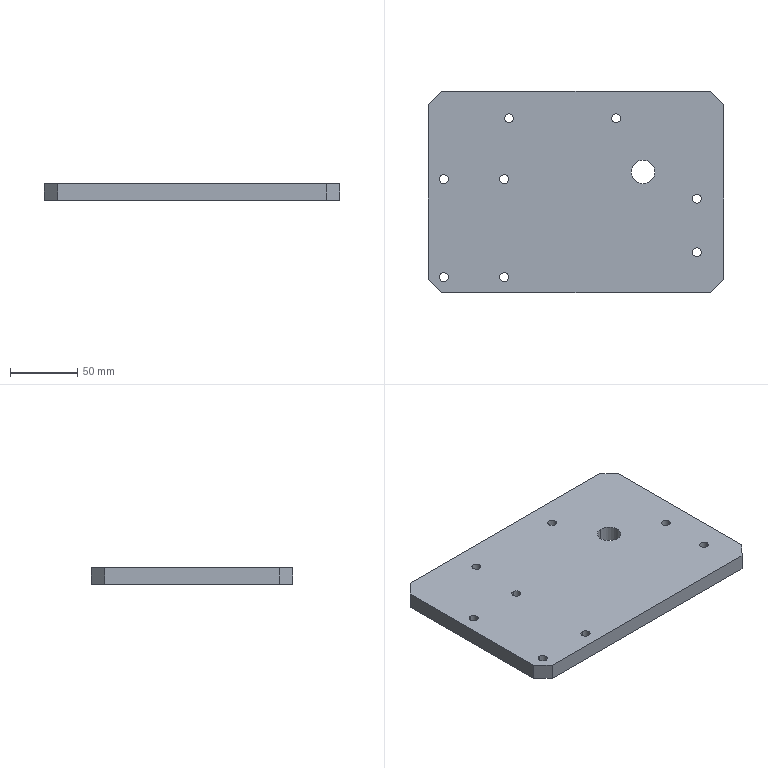Part | SolidWorks | features BaseBody 1 | 1 solid | 40 faces | box 220 x 150 x 12 mm | volume 385674 mm3 | cylinder 26 | plane 14 | commonest cylinder face diameters 6.6 x8 6.8 x8 11 x8 17.5 x2
STEP:
#1=CARTESIAN_POINT('',(349.217,495.647,-547.5));
#2=VERTEX_POINT('',#1);
#3=CARTESIAN_POINT('',(355.817,495.647,-547.5));
#4=VERTEX_POINT('',#3);
#5=CARTESIAN_POINT('',(352.517,495.647,-547.5));
#6=DIRECTION('',(0.,0.,1.));
#7=DIRECTION('',(-1.,0.,0.));
#8=AXIS2_PLACEMENT_3D('',#5,#6,#7);
#9=CIRCLE('',#8,3.3);
#10=EDGE_CURVE('',#2,#4,#9,.T.);
#11=ORIENTED_EDGE('',*,*,#10,.T.);
#12=CARTESIAN_POINT('',(355.817,495.647,-552.7));
#13=VERTEX_POINT('',#12);
#14=CARTESIAN_POINT('',(355.817,495.647,-559.5));
#15=DIRECTION('',(0.,0.,-1.));
#16=VECTOR('',#15,1000.);
#17=LINE('',#14,#16);
#18=EDGE_CURVE('',#4,#13,#17,.T.);
#19=ORIENTED_EDGE('',*,*,#18,.T.);
#20=CARTESIAN_POINT('',(349.217,495.647,-552.7));
#21=VERTEX_POINT('',#20);
#22=CARTESIAN_POINT('',(352.517,495.647,-552.7));
#23=DIRECTION('',(0.,0.,1.));
#24=DIRECTION('',(-1.,0.,0.));
#25=AXIS2_PLACEMENT_3D('',#22,#23,#24);
#26=CIRCLE('',#25,3.3);
#27=EDGE_CURVE('',#21,#13,#26,.T.);
#28=ORIENTED_EDGE('',*,*,#27,.F.);
#29=CARTESIAN_POINT('',(349.217,495.647,-559.5));
#30=DIRECTION('',(0.,0.,-1.));
#31=VECTOR('',#30,1000.);
#32=LINE('',#29,#31);
#33=EDGE_CURVE('',#2,#21,#32,.T.);
#34=ORIENTED_EDGE('',*,*,#33,.F.);
#35=EDGE_LOOP('',(#11,#19,#28,#34));
#36=FACE_OUTER_BOUND('',#35,.T.);
#37=CARTESIAN_POINT('',(352.517,495.647,-559.5));
#38=DIRECTION('',(0.,0.,-1.));
#39=DIRECTION('',(-1.,0.,0.));
#40=AXIS2_PLACEMENT_3D('',#37,#38,#39);
#41=CYLINDRICAL_SURFACE('',#40,3.3);
#42=ADVANCED_FACE('',(#36),#41,.F.);
#43=CARTESIAN_POINT('',(429.217,495.647,-547.5));
#44=VERTEX_POINT('',#43);
#45=CARTESIAN_POINT('',(435.817,495.647,-547.5));
#46=VERTEX_POINT('',#45);
#47=CARTESIAN_POINT('',(432.517,495.647,-547.5));
#48=DIRECTION('',(0.,0.,1.));
#49=DIRECTION('',(-1.,0.,0.));
#50=AXIS2_PLACEMENT_3D('',#47,#48,#49);
#51=CIRCLE('',#50,3.3);
#52=EDGE_CURVE('',#44,#46,#51,.T.);
#53=ORIENTED_EDGE('',*,*,#52,.T.);
#54=CARTESIAN_POINT('',(435.817,495.647,-552.7));
#55=VERTEX_POINT('',#54);
#56=CARTESIAN_POINT('',(435.817,495.647,-559.5));
#57=DIRECTION('',(0.,0.,-1.));
#58=VECTOR('',#57,1000.);
#59=LINE('',#56,#58);
#60=EDGE_CURVE('',#46,#55,#59,.T.);
#61=ORIENTED_EDGE('',*,*,#60,.T.);
#62=CARTESIAN_POINT('',(429.217,495.647,-552.7));
#63=VERTEX_POINT('',#62);
#64=CARTESIAN_POINT('',(432.517,495.647,-552.7));
#65=DIRECTION('',(0.,0.,1.));
#66=DIRECTION('',(-1.,0.,0.));
#67=AXIS2_PLACEMENT_3D('',#64,#65,#66);
#68=CIRCLE('',#67,3.3);
#69=EDGE_CURVE('',#63,#55,#68,.T.);
#70=ORIENTED_EDGE('',*,*,#69,.F.);
#71=CARTESIAN_POINT('',(429.217,495.647,-559.5));
#72=DIRECTION('',(0.,0.,-1.));
#73=VECTOR('',#72,1000.);
#74=LINE('',#71,#73);
#75=EDGE_CURVE('',#44,#63,#74,.T.);
#76=ORIENTED_EDGE('',*,*,#75,.F.);
#77=EDGE_LOOP('',(#53,#61,#70,#76));
#78=FACE_OUTER_BOUND('',#77,.T.);
#79=CARTESIAN_POINT('',(432.517,495.647,-559.5));
#80=DIRECTION('',(0.,0.,-1.));
#81=DIRECTION('',(-1.,0.,0.));
#82=AXIS2_PLACEMENT_3D('',#79,#80,#81);
#83=CYLINDRICAL_SURFACE('',#82,3.3);
#84=ADVANCED_FACE('',(#78),#83,.F.);
#85=CARTESIAN_POINT('',(489.217,395.647,-547.5));
#86=VERTEX_POINT('',#85);
#87=CARTESIAN_POINT('',(495.817,395.647,-547.5));
#88=VERTEX_POINT('',#87);
#89=CARTESIAN_POINT('',(492.517,395.647,-547.5));
#90=DIRECTION('',(0.,0.,1.));
#91=DIRECTION('',(-1.,0.,0.));
#92=AXIS2_PLACEMENT_3D('',#89,#90,#91);
#93=CIRCLE('',#92,3.3);
#94=EDGE_CURVE('',#86,#88,#93,.T.);
#95=ORIENTED_EDGE('',*,*,#94,.T.);
#96=CARTESIAN_POINT('',(495.817,395.647,-552.7));
#97=VERTEX_POINT('',#96);
#98=CARTESIAN_POINT('',(495.817,395.647,-559.5));
#99=DIRECTION('',(0.,0.,-1.));
#100=VECTOR('',#99,1000.);
#101=LINE('',#98,#100);
#102=EDGE_CURVE('',#88,#97,#101,.T.);
#103=ORIENTED_EDGE('',*,*,#102,.T.);
#104=CARTESIAN_POINT('',(489.217,395.647,-552.7));
#105=VERTEX_POINT('',#104);
#106=CARTESIAN_POINT('',(492.517,395.647,-552.7));
#107=DIRECTION('',(0.,0.,1.));
#108=DIRECTION('',(-1.,0.,0.));
#109=AXIS2_PLACEMENT_3D('',#106,#107,#108);
#110=CIRCLE('',#109,3.3);
#111=EDGE_CURVE('',#105,#97,#110,.T.);
#112=ORIENTED_EDGE('',*,*,#111,.F.);
#113=CARTESIAN_POINT('',(489.217,395.647,-559.5));
#114=DIRECTION('',(0.,0.,-1.));
#115=VECTOR('',#114,1000.);
#116=LINE('',#113,#115);
#117=EDGE_CURVE('',#86,#105,#116,.T.);
#118=ORIENTED_EDGE('',*,*,#117,.F.);
#119=EDGE_LOOP('',(#95,#103,#112,#118));
#120=FACE_OUTER_BOUND('',#119,.T.);
#121=CARTESIAN_POINT('',(492.517,395.647,-559.5));
#122=DIRECTION('',(0.,0.,-1.));
#123=DIRECTION('',(-1.,0.,0.));
#124=AXIS2_PLACEMENT_3D('',#121,#122,#123);
#125=CYLINDRICAL_SURFACE('',#124,3.3);
#126=ADVANCED_FACE('',(#120),#125,.F.);
#127=CARTESIAN_POINT('',(489.217,435.647,-547.5));
#128=VERTEX_POINT('',#127);
#129=CARTESIAN_POINT('',(495.817,435.647,-547.5));
#130=VERTEX_POINT('',#129);
#131=CARTESIAN_POINT('',(492.517,435.647,-547.5));
#132=DIRECTION('',(0.,0.,1.));
#133=DIRECTION('',(-1.,0.,0.));
#134=AXIS2_PLACEMENT_3D('',#131,#132,#133);
#135=CIRCLE('',#134,3.3);
#136=EDGE_CURVE('',#128,#130,#135,.T.);
#137=ORIENTED_EDGE('',*,*,#136,.T.);
#138=CARTESIAN_POINT('',(495.817,435.647,-552.7));
#139=VERTEX_POINT('',#138);
#140=CARTESIAN_POINT('',(495.817,435.647,-559.5));
#141=DIRECTION('',(0.,0.,-1.));
#142=VECTOR('',#141,1000.);
#143=LINE('',#140,#142);
#144=EDGE_CURVE('',#130,#139,#143,.T.);
#145=ORIENTED_EDGE('',*,*,#144,.T.);
#146=CARTESIAN_POINT('',(489.217,435.647,-552.7));
#147=VERTEX_POINT('',#146);
#148=CARTESIAN_POINT('',(492.517,435.647,-552.7));
#149=DIRECTION('',(0.,0.,1.));
#150=DIRECTION('',(-1.,0.,0.));
#151=AXIS2_PLACEMENT_3D('',#148,#149,#150);
#152=CIRCLE('',#151,3.3);
#153=EDGE_CURVE('',#147,#139,#152,.T.);
#154=ORIENTED_EDGE('',*,*,#153,.F.);
#155=CARTESIAN_POINT('',(489.217,435.647,-559.5));
#156=DIRECTION('',(0.,0.,-1.));
#157=VECTOR('',#156,1000.);
#158=LINE('',#155,#157);
#159=EDGE_CURVE('',#128,#147,#158,.T.);
#160=ORIENTED_EDGE('',*,*,#159,.F.);
#161=EDGE_LOOP('',(#137,#145,#154,#160));
#162=FACE_OUTER_BOUND('',#161,.T.);
#163=CARTESIAN_POINT('',(492.517,435.647,-559.5));
#164=DIRECTION('',(0.,0.,-1.));
#165=DIRECTION('',(-1.,0.,0.));
#166=AXIS2_PLACEMENT_3D('',#163,#164,#165);
#167=CYLINDRICAL_SURFACE('',#166,3.3);
#168=ADVANCED_FACE('',(#162),#167,.F.);
#169=CARTESIAN_POINT('',(452.517,464.397,-547.5));
#170=VERTEX_POINT('',#169);
#171=CARTESIAN_POINT('',(452.517,446.897,-547.5));
#172=VERTEX_POINT('',#171);
#173=CARTESIAN_POINT('',(452.517,455.647,-547.5));
#174=DIRECTION('',(0.,0.,1.));
#175=DIRECTION('',(0.,1.,0.));
#176=AXIS2_PLACEMENT_3D('',#173,#174,#175);
#177=CIRCLE('',#176,8.75);
#178=EDGE_CURVE('',#170,#172,#177,.T.);
#179=ORIENTED_EDGE('',*,*,#178,.T.);
#180=CARTESIAN_POINT('',(452.517,446.897,-559.5));
#181=VERTEX_POINT('',#180);
#182=CARTESIAN_POINT('',(452.517,446.897,-559.5));
#183=DIRECTION('',(0.,0.,-1.));
#184=VECTOR('',#183,1000.);
#185=LINE('',#182,#184);
#186=EDGE_CURVE('',#172,#181,#185,.T.);
#187=ORIENTED_EDGE('',*,*,#186,.T.);
#188=CARTESIAN_POINT('',(452.517,464.397,-559.5));
#189=VERTEX_POINT('',#188);
#190=CARTESIAN_POINT('',(452.517,455.647,-559.5));
#191=DIRECTION('',(0.,0.,1.));
#192=DIRECTION('',(0.,1.,0.));
#193=AXIS2_PLACEMENT_3D('',#190,#191,#192);
#194=CIRCLE('',#193,8.75);
#195=EDGE_CURVE('',#189,#181,#194,.T.);
#196=ORIENTED_EDGE('',*,*,#195,.F.);
#197=CARTESIAN_POINT('',(452.517,464.397,-559.5));
#198=DIRECTION('',(0.,0.,-1.));
#199=VECTOR('',#198,1000.);
#200=LINE('',#197,#199);
#201=EDGE_CURVE('',#170,#189,#200,.T.);
#202=ORIENTED_EDGE('',*,*,#201,.F.);
#203=EDGE_LOOP('',(#179,#187,#196,#202));
#204=FACE_OUTER_BOUND('',#203,.T.);
#205=CARTESIAN_POINT('',(452.517,455.647,-559.5));
#206=DIRECTION('',(0.,0.,-1.));
#207=DIRECTION('',(0.,1.,0.));
#208=AXIS2_PLACEMENT_3D('',#205,#206,#207);
#209=CYLINDRICAL_SURFACE('',#208,8.75);
#210=ADVANCED_FACE('',(#204),#209,.F.);
#211=CARTESIAN_POINT('',(304.017,380.547,-547.5));
#212=VERTEX_POINT('',#211);
#213=CARTESIAN_POINT('',(304.017,373.747,-547.5));
#214=VERTEX_POINT('',#213);
#215=CARTESIAN_POINT('',(304.017,377.147,-547.5));
#216=DIRECTION('',(0.,0.,1.));
#217=DIRECTION('',(0.,1.,0.));
#218=AXIS2_PLACEMENT_3D('',#215,#216,#217);
#219=CIRCLE('',#218,3.4);
#220=EDGE_CURVE('',#212,#214,#219,.T.);
#221=ORIENTED_EDGE('',*,*,#220,.T.);
#222=CARTESIAN_POINT('',(304.017,373.747,-559.5));
#223=VERTEX_POINT('',#222);
#224=CARTESIAN_POINT('',(304.017,373.747,-559.5));
#225=DIRECTION('',(0.,0.,-1.));
#226=VECTOR('',#225,1000.);
#227=LINE('',#224,#226);
#228=EDGE_CURVE('',#214,#223,#227,.T.);
#229=ORIENTED_EDGE('',*,*,#228,.T.);
#230=CARTESIAN_POINT('',(304.017,380.547,-559.5));
#231=VERTEX_POINT('',#230);
#232=CARTESIAN_POINT('',(304.017,377.147,-559.5));
#233=DIRECTION('',(0.,0.,1.));
#234=DIRECTION('',(0.,1.,0.));
#235=AXIS2_PLACEMENT_3D('',#232,#233,#234);
#236=CIRCLE('',#235,3.4);
#237=EDGE_CURVE('',#231,#223,#236,.T.);
#238=ORIENTED_EDGE('',*,*,#237,.F.);
#239=CARTESIAN_POINT('',(304.017,380.547,-559.5));
#240=DIRECTION('',(0.,0.,-1.));
#241=VECTOR('',#240,1000.);
#242=LINE('',#239,#241);
#243=EDGE_CURVE('',#212,#231,#242,.T.);
#244=ORIENTED_EDGE('',*,*,#243,.F.);
#245=EDGE_LOOP('',(#221,#229,#238,#244));
#246=FACE_OUTER_BOUND('',#245,.T.);
#247=CARTESIAN_POINT('',(304.017,377.147,-559.5));
#248=DIRECTION('',(0.,0.,-1.));
#249=DIRECTION('',(0.,1.,0.));
#250=AXIS2_PLACEMENT_3D('',#247,#248,#249);
#251=CYLINDRICAL_SURFACE('',#250,3.4);
#252=ADVANCED_FACE('',(#246),#251,.F.);
#253=CARTESIAN_POINT('',(349.017,380.547,-547.5));
#254=VERTEX_POINT('',#253);
#255=CARTESIAN_POINT('',(349.017,373.747,-547.5));
#256=VERTEX_POINT('',#255);
#257=CARTESIAN_POINT('',(349.017,377.147,-547.5));
#258=DIRECTION('',(0.,0.,1.));
#259=DIRECTION('',(0.,1.,0.));
#260=AXIS2_PLACEMENT_3D('',#257,#258,#259);
#261=CIRCLE('',#260,3.4);
#262=EDGE_CURVE('',#254,#256,#261,.T.);
#263=ORIENTED_EDGE('',*,*,#262,.T.);
#264=CARTESIAN_POINT('',(349.017,373.747,-559.5));
#265=VERTEX_POINT('',#264);
#266=CARTESIAN_POINT('',(349.017,373.747,-559.5));
#267=DIRECTION('',(0.,0.,-1.));
#268=VECTOR('',#267,1000.);
#269=LINE('',#266,#268);
#270=EDGE_CURVE('',#256,#265,#269,.T.);
#271=ORIENTED_EDGE('',*,*,#270,.T.);
#272=CARTESIAN_POINT('',(349.017,380.547,-559.5));
#273=VERTEX_POINT('',#272);
#274=CARTESIAN_POINT('',(349.017,377.147,-559.5));
#275=DIRECTION('',(0.,0.,1.));
#276=DIRECTION('',(0.,1.,0.));
#277=AXIS2_PLACEMENT_3D('',#274,#275,#276);
#278=CIRCLE('',#277,3.4);
#279=EDGE_CURVE('',#273,#265,#278,.T.);
#280=ORIENTED_EDGE('',*,*,#279,.F.);
#281=CARTESIAN_POINT('',(349.017,380.547,-559.5));
#282=DIRECTION('',(0.,0.,-1.));
#283=VECTOR('',#282,1000.);
#284=LINE('',#281,#283);
#285=EDGE_CURVE('',#254,#273,#284,.T.);
#286=ORIENTED_EDGE('',*,*,#285,.F.);
#287=EDGE_LOOP('',(#263,#271,#280,#286));
#288=FACE_OUTER_BOUND('',#287,.T.);
#289=CARTESIAN_POINT('',(349.017,377.147,-559.5));
#290=DIRECTION('',(0.,0.,-1.));
#291=DIRECTION('',(0.,1.,0.));
#292=AXIS2_PLACEMENT_3D('',#289,#290,#291);
#293=CYLINDRICAL_SURFACE('',#292,3.4);
#294=ADVANCED_FACE('',(#288),#293,.F.);
#295=CARTESIAN_POINT('',(304.017,453.547,-547.5));
#296=VERTEX_POINT('',#295);
#297=CARTESIAN_POINT('',(304.017,446.747,-547.5));
#298=VERTEX_POINT('',#297);
#299=CARTESIAN_POINT('',(304.017,450.147,-547.5));
#300=DIRECTION('',(0.,0.,1.));
#301=DIRECTION('',(0.,1.,0.));
#302=AXIS2_PLACEMENT_3D('',#299,#300,#301);
#303=CIRCLE('',#302,3.4);
#304=EDGE_CURVE('',#296,#298,#303,.T.);
#305=ORIENTED_EDGE('',*,*,#304,.T.);
#306=CARTESIAN_POINT('',(304.017,446.747,-559.5));
#307=VERTEX_POINT('',#306);
#308=CARTESIAN_POINT('',(304.017,446.747,-559.5));
#309=DIRECTION('',(0.,0.,-1.));
#310=VECTOR('',#309,1000.);
#311=LINE('',#308,#310);
#312=EDGE_CURVE('',#298,#307,#311,.T.);
#313=ORIENTED_EDGE('',*,*,#312,.T.);
#314=CARTESIAN_POINT('',(304.017,453.547,-559.5));
#315=VERTEX_POINT('',#314);
#316=CARTESIAN_POINT('',(304.017,450.147,-559.5));
#317=DIRECTION('',(0.,0.,1.));
#318=DIRECTION('',(0.,1.,0.));
#319=AXIS2_PLACEMENT_3D('',#316,#317,#318);
#320=CIRCLE('',#319,3.4);
#321=EDGE_CURVE('',#315,#307,#320,.T.);
#322=ORIENTED_EDGE('',*,*,#321,.F.);
#323=CARTESIAN_POINT('',(304.017,453.547,-559.5));
#324=DIRECTION('',(0.,0.,-1.));
#325=VECTOR('',#324,1000.);
#326=LINE('',#323,#325);
#327=EDGE_CURVE('',#296,#315,#326,.T.);
#328=ORIENTED_EDGE('',*,*,#327,.F.);
#329=EDGE_LOOP('',(#305,#313,#322,#328));
#330=FACE_OUTER_BOUND('',#329,.T.);
#331=CARTESIAN_POINT('',(304.017,450.147,-559.5));
#332=DIRECTION('',(0.,0.,-1.));
#333=DIRECTION('',(0.,1.,0.));
#334=AXIS2_PLACEMENT_3D('',#331,#332,#333);
#335=CYLINDRICAL_SURFACE('',#334,3.4);
#336=ADVANCED_FACE('',(#330),#335,.F.);
#337=CARTESIAN_POINT('',(349.017,453.547,-547.5));
#338=VERTEX_POINT('',#337);
#339=CARTESIAN_POINT('',(349.017,446.747,-547.5));
#340=VERTEX_POINT('',#339);
#341=CARTESIAN_POINT('',(349.017,450.147,-547.5));
#342=DIRECTION('',(0.,0.,1.));
#343=DIRECTION('',(0.,1.,0.));
#344=AXIS2_PLACEMENT_3D('',#341,#342,#343);
#345=CIRCLE('',#344,3.4);
#346=EDGE_CURVE('',#338,#340,#345,.T.);
#347=ORIENTED_EDGE('',*,*,#346,.T.);
#348=CARTESIAN_POINT('',(349.017,446.747,-559.5));
#349=VERTEX_POINT('',#348);
#350=CARTESIAN_POINT('',(349.017,446.747,-559.5));
#351=DIRECTION('',(0.,0.,-1.));
#352=VECTOR('',#351,1000.);
#353=LINE('',#350,#352);
#354=EDGE_CURVE('',#340,#349,#353,.T.);
#355=ORIENTED_EDGE('',*,*,#354,.T.);
#356=CARTESIAN_POINT('',(349.017,453.547,-559.5));
#357=VERTEX_POINT('',#356);
#358=CARTESIAN_POINT('',(349.017,450.147,-559.5));
#359=DIRECTION('',(0.,0.,1.));
#360=DIRECTION('',(0.,1.,0.));
#361=AXIS2_PLACEMENT_3D('',#358,#359,#360);
#362=CIRCLE('',#361,3.4);
#363=EDGE_CURVE('',#357,#349,#362,.T.);
#364=ORIENTED_EDGE('',*,*,#363,.F.);
#365=CARTESIAN_POINT('',(349.017,453.547,-559.5));
#366=DIRECTION('',(0.,0.,-1.));
#367=VECTOR('',#366,1000.);
#368=LINE('',#365,#367);
#369=EDGE_CURVE('',#338,#357,#368,.T.);
#370=ORIENTED_EDGE('',*,*,#369,.F.);
#371=EDGE_LOOP('',(#347,#355,#364,#370));
#372=FACE_OUTER_BOUND('',#371,.T.);
#373=CARTESIAN_POINT('',(349.017,450.147,-559.5));
#374=DIRECTION('',(0.,0.,-1.));
#375=DIRECTION('',(0.,1.,0.));
#376=AXIS2_PLACEMENT_3D('',#373,#374,#375);
#377=CYLINDRICAL_SURFACE('',#376,3.4);
#378=ADVANCED_FACE('',(#372),#377,.F.);
#379=CARTESIAN_POINT('',(347.017,495.647,-552.7));
#380=VERTEX_POINT('',#379);
#381=CARTESIAN_POINT('',(358.017,495.647,-552.7));
#382=VERTEX_POINT('',#381);
#383=CARTESIAN_POINT('',(352.517,495.647,-552.7));
#384=DIRECTION('',(0.,0.,1.));
#385=DIRECTION('',(-1.,0.,0.));
#386=AXIS2_PLACEMENT_3D('',#383,#384,#385);
#387=CIRCLE('',#386,5.5);
#388=EDGE_CURVE('',#380,#382,#387,.T.);
#389=ORIENTED_EDGE('',*,*,#388,.T.);
#390=CARTESIAN_POINT('',(358.017,495.647,-559.5));
#391=VERTEX_POINT('',#390);
#392=CARTESIAN_POINT('',(358.017,495.647,-559.5));
#393=DIRECTION('',(0.,0.,-1.));
#394=VECTOR('',#393,1000.);
#395=LINE('',#392,#394);
#396=EDGE_CURVE('',#382,#391,#395,.T.);
#397=ORIENTED_EDGE('',*,*,#396,.T.);
#398=CARTESIAN_POINT('',(347.017,495.647,-559.5));
#399=VERTEX_POINT('',#398);
#400=CARTESIAN_POINT('',(352.517,495.647,-559.5));
#401=DIRECTION('',(0.,0.,1.));
#402=DIRECTION('',(-1.,0.,0.));
#403=AXIS2_PLACEMENT_3D('',#400,#401,#402);
#404=CIRCLE('',#403,5.5);
#405=EDGE_CURVE('',#399,#391,#404,.T.);
#406=ORIENTED_EDGE('',*,*,#405,.F.);
#407=CARTESIAN_POINT('',(347.017,495.647,-559.5));
#408=DIRECTION('',(0.,0.,-1.));
#409=VECTOR('',#408,1000.);
#410=LINE('',#407,#409);
#411=EDGE_CURVE('',#380,#399,#410,.T.);
#412=ORIENTED_EDGE('',*,*,#411,.F.);
#413=EDGE_LOOP('',(#389,#397,#406,#412));
#414=FACE_OUTER_BOUND('',#413,.T.);
#415=CARTESIAN_POINT('',(352.517,495.647,-559.5));
#416=DIRECTION('',(0.,0.,-1.));
#417=DIRECTION('',(-1.,0.,0.));
#418=AXIS2_PLACEMENT_3D('',#415,#416,#417);
#419=CYLINDRICAL_SURFACE('',#418,5.5);
#420=ADVANCED_FACE('',(#414),#419,.F.);
#421=CARTESIAN_POINT('',(427.017,495.647,-552.7));
#422=VERTEX_POINT('',#421);
#423=CARTESIAN_POINT('',(438.017,495.647,-552.7));
#424=VERTEX_POINT('',#423);
#425=CARTESIAN_POINT('',(432.517,495.647,-552.7));
#426=DIRECTION('',(0.,0.,1.));
#427=DIRECTION('',(-1.,0.,0.));
#428=AXIS2_PLACEMENT_3D('',#425,#426,#427);
#429=CIRCLE('',#428,5.5);
#430=EDGE_CURVE('',#422,#424,#429,.T.);
#431=ORIENTED_EDGE('',*,*,#430,.T.);
#432=CARTESIAN_POINT('',(438.017,495.647,-559.5));
#433=VERTEX_POINT('',#432);
#434=CARTESIAN_POINT('',(438.017,495.647,-559.5));
#435=DIRECTION('',(0.,0.,-1.));
#436=VECTOR('',#435,1000.);
#437=LINE('',#434,#436);
#438=EDGE_CURVE('',#424,#433,#437,.T.);
#439=ORIENTED_EDGE('',*,*,#438,.T.);
#440=CARTESIAN_POINT('',(427.017,495.647,-559.5));
#441=VERTEX_POINT('',#440);
#442=CARTESIAN_POINT('',(432.517,495.647,-559.5));
#443=DIRECTION('',(0.,0.,1.));
#444=DIRECTION('',(-1.,0.,0.));
#445=AXIS2_PLACEMENT_3D('',#442,#443,#444);
#446=CIRCLE('',#445,5.5);
#447=EDGE_CURVE('',#441,#433,#446,.T.);
#448=ORIENTED_EDGE('',*,*,#447,.F.);
#449=CARTESIAN_POINT('',(427.017,495.647,-559.5));
#450=DIRECTION('',(0.,0.,-1.));
#451=VECTOR('',#450,1000.);
#452=LINE('',#449,#451);
#453=EDGE_CURVE('',#422,#441,#452,.T.);
#454=ORIENTED_EDGE('',*,*,#453,.F.);
#455=EDGE_LOOP('',(#431,#439,#448,#454));
#456=FACE_OUTER_BOUND('',#455,.T.);
#457=CARTESIAN_POINT('',(432.517,495.647,-559.5));
#458=DIRECTION('',(0.,0.,-1.));
#459=DIRECTION('',(-1.,0.,0.));
#460=AXIS2_PLACEMENT_3D('',#457,#458,#459);
#461=CYLINDRICAL_SURFACE('',#460,5.5);
#462=ADVANCED_FACE('',(#456),#461,.F.);
#463=CARTESIAN_POINT('',(487.017,395.647,-552.7));
#464=VERTEX_POINT('',#463);
#465=CARTESIAN_POINT('',(498.017,395.647,-552.7));
#466=VERTEX_POINT('',#465);
#467=CARTESIAN_POINT('',(492.517,395.647,-552.7));
#468=DIRECTION('',(0.,0.,1.));
#469=DIRECTION('',(-1.,0.,0.));
#470=AXIS2_PLACEMENT_3D('',#467,#468,#469);
#471=CIRCLE('',#470,5.5);
#472=EDGE_CURVE('',#464,#466,#471,.T.);
#473=ORIENTED_EDGE('',*,*,#472,.T.);
#474=CARTESIAN_POINT('',(498.017,395.647,-559.5));
#475=VERTEX_POINT('',#474);
#476=CARTESIAN_POINT('',(498.017,395.647,-559.5));
#477=DIRECTION('',(0.,0.,-1.));
#478=VECTOR('',#477,1000.);
#479=LINE('',#476,#478);
#480=EDGE_CURVE('',#466,#475,#479,.T.);
#481=ORIENTED_EDGE('',*,*,#480,.T.);
#482=CARTESIAN_POINT('',(487.017,395.647,-559.5));
#483=VERTEX_POINT('',#482);
#484=CARTESIAN_POINT('',(492.517,395.647,-559.5));
#485=DIRECTION('',(0.,0.,1.));
#486=DIRECTION('',(-1.,0.,0.));
#487=AXIS2_PLACEMENT_3D('',#484,#485,#486);
#488=CIRCLE('',#487,5.5);
#489=EDGE_CURVE('',#483,#475,#488,.T.);
#490=ORIENTED_EDGE('',*,*,#489,.F.);
#491=CARTESIAN_POINT('',(487.017,395.647,-559.5));
#492=DIRECTION('',(0.,0.,-1.));
#493=VECTOR('',#492,1000.);
#494=LINE('',#491,#493);
#495=EDGE_CURVE('',#464,#483,#494,.T.);
#496=ORIENTED_EDGE('',*,*,#495,.F.);
#497=EDGE_LOOP('',(#473,#481,#490,#496));
#498=FACE_OUTER_BOUND('',#497,.T.);
#499=CARTESIAN_POINT('',(492.517,395.647,-559.5));
#500=DIRECTION('',(0.,0.,-1.));
#501=DIRECTION('',(-1.,0.,0.));
#502=AXIS2_PLACEMENT_3D('',#499,#500,#501);
#503=CYLINDRICAL_SURFACE('',#502,5.5);
#504=ADVANCED_FACE('',(#498),#503,.F.);
#505=CARTESIAN_POINT('',(487.017,435.647,-552.7));
#506=VERTEX_POINT('',#505);
#507=CARTESIAN_POINT('',(498.017,435.647,-552.7));
#508=VERTEX_POINT('',#507);
#509=CARTESIAN_POINT('',(492.517,435.647,-552.7));
#510=DIRECTION('',(0.,0.,1.));
#511=DIRECTION('',(-1.,0.,0.));
#512=AXIS2_PLACEMENT_3D('',#509,#510,#511);
#513=CIRCLE('',#512,5.5);
#514=EDGE_CURVE('',#506,#508,#513,.T.);
#515=ORIENTED_EDGE('',*,*,#514,.T.);
#516=CARTESIAN_POINT('',(498.017,435.647,-559.5));
#517=VERTEX_POINT('',#516);
#518=CARTESIAN_POINT('',(498.017,435.647,-559.5));
#519=DIRECTION('',(0.,0.,-1.));
#520=VECTOR('',#519,1000.);
#521=LINE('',#518,#520);
#522=EDGE_CURVE('',#508,#517,#521,.T.);
#523=ORIENTED_EDGE('',*,*,#522,.T.);
#524=CARTESIAN_POINT('',(487.017,435.647,-559.5));
#525=VERTEX_POINT('',#524);
#526=CARTESIAN_POINT('',(492.517,435.647,-559.5));
#527=DIRECTION('',(0.,0.,1.));
#528=DIRECTION('',(-1.,0.,0.));
#529=AXIS2_PLACEMENT_3D('',#526,#527,#528);
#530=CIRCLE('',#529,5.5);
#531=EDGE_CURVE('',#525,#517,#530,.T.);
#532=ORIENTED_EDGE('',*,*,#531,.F.);
#533=CARTESIAN_POINT('',(487.017,435.647,-559.5));
#534=DIRECTION('',(0.,0.,-1.));
#535=VECTOR('',#534,1000.);
#536=LINE('',#533,#535);
#537=EDGE_CURVE('',#506,#525,#536,.T.);
#538=ORIENTED_EDGE('',*,*,#537,.F.);
#539=EDGE_LOOP('',(#515,#523,#532,#538));
#540=FACE_OUTER_BOUND('',#539,.T.);
#541=CARTESIAN_POINT('',(492.517,435.647,-559.5));
#542=DIRECTION('',(0.,0.,-1.));
#543=DIRECTION('',(-1.,0.,0.));
#544=AXIS2_PLACEMENT_3D('',#541,#542,#543);
#545=CYLINDRICAL_SURFACE('',#544,5.5);
#546=ADVANCED_FACE('',(#540),#545,.F.);
#547=CARTESIAN_POINT('',(512.517,375.647,-547.5));
#548=VERTEX_POINT('',#547);
#549=CARTESIAN_POINT('',(502.517,365.647,-547.5));
#550=VERTEX_POINT('',#549);
#551=CARTESIAN_POINT('',(512.517,375.647,-547.5));
#552=DIRECTION('',(-0.7071,-0.7071,0.));
#553=VECTOR('',#552,1000.);
#554=LINE('',#551,#553);
#555=EDGE_CURVE('',#548,#550,#554,.T.);
#556=ORIENTED_EDGE('',*,*,#555,.F.);
#557=CARTESIAN_POINT('',(512.517,505.647,-547.5));
#558=VERTEX_POINT('',#557);
#559=CARTESIAN_POINT('',(512.517,0.,-547.5));
#560=DIRECTION('',(0.,-1.,0.));
#561=VECTOR('',#560,1000.);
#562=LINE('',#559,#561);
#563=EDGE_CURVE('',#558,#548,#562,.T.);
#564=ORIENTED_EDGE('',*,*,#563,.F.);
#565=CARTESIAN_POINT('',(502.517,515.647,-547.5));
#566=VERTEX_POINT('',#565);
#567=CARTESIAN_POINT('',(502.517,515.647,-547.5));
#568=DIRECTION('',(0.7071,-0.7071,0.));
#569=VECTOR('',#568,1000.);
#570=LINE('',#567,#569);
#571=EDGE_CURVE('',#566,#558,#570,.T.);
#572=ORIENTED_EDGE('',*,*,#571,.F.);
#573=CARTESIAN_POINT('',(302.517,515.647,-547.5));
#574=VERTEX_POINT('',#573);
#575=CARTESIAN_POINT('',(0.,515.647,-547.5));
#576=DIRECTION('',(1.,0.,0.));
#577=VECTOR('',#576,1000.);
#578=LINE('',#575,#577);
#579=EDGE_CURVE('',#574,#566,#578,.T.);
#580=ORIENTED_EDGE('',*,*,#579,.F.);
#581=CARTESIAN_POINT('',(292.517,505.647,-547.5));
#582=VERTEX_POINT('',#581);
#583=CARTESIAN_POINT('',(292.517,505.647,-547.5));
#584=DIRECTION('',(0.7071,0.7071,0.));
#585=VECTOR('',#584,1000.);
#586=LINE('',#583,#585);
#587=EDGE_CURVE('',#582,#574,#586,.T.);
#588=ORIENTED_EDGE('',*,*,#587,.F.);
#589=CARTESIAN_POINT('',(292.517,375.647,-547.5));
#590=VERTEX_POINT('',#589);
#591=CARTESIAN_POINT('',(292.517,0.,-547.5));
#592=DIRECTION('',(0.,1.,0.));
#593=VECTOR('',#592,1000.);
#594=LINE('',#591,#593);
#595=EDGE_CURVE('',#590,#582,#594,.T.);
#596=ORIENTED_EDGE('',*,*,#595,.F.);
#597=CARTESIAN_POINT('',(302.517,365.647,-547.5));
#598=VERTEX_POINT('',#597);
#599=CARTESIAN_POINT('',(302.517,365.647,-547.5));
#600=DIRECTION('',(-0.7071,0.7071,0.));
#601=VECTOR('',#600,1000.);
#602=LINE('',#599,#601);
#603=EDGE_CURVE('',#598,#590,#602,.T.);
#604=ORIENTED_EDGE('',*,*,#603,.F.);
#605=CARTESIAN_POINT('',(0.,365.647,-547.5));
#606=DIRECTION('',(-1.,0.,0.));
#607=VECTOR('',#606,1000.);
#608=LINE('',#605,#607);
#609=EDGE_CURVE('',#550,#598,#608,.T.);
#610=ORIENTED_EDGE('',*,*,#609,.F.);
#611=EDGE_LOOP('',(#556,#564,#572,#580,#588,#596,#604,#610));
#612=FACE_OUTER_BOUND('',#611,.T.);
#613=ORIENTED_EDGE('',*,*,#10,.F.);
#614=CARTESIAN_POINT('',(352.517,495.647,-547.5));
#615=DIRECTION('',(0.,0.,1.));
#616=DIRECTION('',(-1.,0.,0.));
#617=AXIS2_PLACEMENT_3D('',#614,#615,#616);
#618=CIRCLE('',#617,3.3);
#619=EDGE_CURVE('',#4,#2,#618,.T.);
#620=ORIENTED_EDGE('',*,*,#619,.F.);
#621=EDGE_LOOP('',(#613,#620));
#622=FACE_BOUND('',#621,.T.);
#623=ORIENTED_EDGE('',*,*,#52,.F.);
#624=CARTESIAN_POINT('',(432.517,495.647,-547.5));
#625=DIRECTION('',(0.,0.,1.));
#626=DIRECTION('',(-1.,0.,0.));
#627=AXIS2_PLACEMENT_3D('',#624,#625,#626);
#628=CIRCLE('',#627,3.3);
#629=EDGE_CURVE('',#46,#44,#628,.T.);
#630=ORIENTED_EDGE('',*,*,#629,.F.);
#631=EDGE_LOOP('',(#623,#630));
#632=FACE_BOUND('',#631,.T.);
#633=ORIENTED_EDGE('',*,*,#94,.F.);
#634=CARTESIAN_POINT('',(492.517,395.647,-547.5));
#635=DIRECTION('',(0.,0.,1.));
#636=DIRECTION('',(-1.,0.,0.));
#637=AXIS2_PLACEMENT_3D('',#634,#635,#636);
#638=CIRCLE('',#637,3.3);
#639=EDGE_CURVE('',#88,#86,#638,.T.);
#640=ORIENTED_EDGE('',*,*,#639,.F.);
#641=EDGE_LOOP('',(#633,#640));
#642=FACE_BOUND('',#641,.T.);
#643=ORIENTED_EDGE('',*,*,#136,.F.);
#644=CARTESIAN_POINT('',(492.517,435.647,-547.5));
#645=DIRECTION('',(0.,0.,1.));
#646=DIRECTION('',(-1.,0.,0.));
#647=AXIS2_PLACEMENT_3D('',#644,#645,#646);
#648=CIRCLE('',#647,3.3);
#649=EDGE_CURVE('',#130,#128,#648,.T.);
#650=ORIENTED_EDGE('',*,*,#649,.F.);
#651=EDGE_LOOP('',(#643,#650));
#652=FACE_BOUND('',#651,.T.);
#653=ORIENTED_EDGE('',*,*,#178,.F.);
#654=CARTESIAN_POINT('',(452.517,455.647,-547.5));
#655=DIRECTION('',(0.,0.,1.));
#656=DIRECTION('',(0.,1.,0.));
#657=AXIS2_PLACEMENT_3D('',#654,#655,#656);
#658=CIRCLE('',#657,8.75);
#659=EDGE_CURVE('',#172,#170,#658,.T.);
#660=ORIENTED_EDGE('',*,*,#659,.F.);
#661=EDGE_LOOP('',(#653,#660));
#662=FACE_BOUND('',#661,.T.);
#663=ORIENTED_EDGE('',*,*,#220,.F.);
#664=CARTESIAN_POINT('',(304.017,377.147,-547.5));
#665=DIRECTION('',(0.,0.,1.));
#666=DIRECTION('',(0.,1.,0.));
#667=AXIS2_PLACEMENT_3D('',#664,#665,#666);
#668=CIRCLE('',#667,3.4);
#669=EDGE_CURVE('',#214,#212,#668,.T.);
#670=ORIENTED_EDGE('',*,*,#669,.F.);
#671=EDGE_LOOP('',(#663,#670));
#672=FACE_BOUND('',#671,.T.);
#673=ORIENTED_EDGE('',*,*,#262,.F.);
#674=CARTESIAN_POINT('',(349.017,377.147,-547.5));
#675=DIRECTION('',(0.,0.,1.));
#676=DIRECTION('',(0.,1.,0.));
#677=AXIS2_PLACEMENT_3D('',#674,#675,#676);
#678=CIRCLE('',#677,3.4);
#679=EDGE_CURVE('',#256,#254,#678,.T.);
#680=ORIENTED_EDGE('',*,*,#679,.F.);
#681=EDGE_LOOP('',(#673,#680));
#682=FACE_BOUND('',#681,.T.);
#683=ORIENTED_EDGE('',*,*,#304,.F.);
#684=CARTESIAN_POINT('',(304.017,450.147,-547.5));
#685=DIRECTION('',(0.,0.,1.));
#686=DIRECTION('',(0.,1.,0.));
#687=AXIS2_PLACEMENT_3D('',#684,#685,#686);
#688=CIRCLE('',#687,3.4);
#689=EDGE_CURVE('',#298,#296,#688,.T.);
#690=ORIENTED_EDGE('',*,*,#689,.F.);
#691=EDGE_LOOP('',(#683,#690));
#692=FACE_BOUND('',#691,.T.);
#693=ORIENTED_EDGE('',*,*,#346,.F.);
#694=CARTESIAN_POINT('',(349.017,450.147,-547.5));
#695=DIRECTION('',(0.,0.,1.));
#696=DIRECTION('',(0.,1.,0.));
#697=AXIS2_PLACEMENT_3D('',#694,#695,#696);
#698=CIRCLE('',#697,3.4);
#699=EDGE_CURVE('',#340,#338,#698,.T.);
#700=ORIENTED_EDGE('',*,*,#699,.F.);
#701=EDGE_LOOP('',(#693,#700));
#702=FACE_BOUND('',#701,.T.);
#703=CARTESIAN_POINT('',(0.,0.,-547.5));
#704=DIRECTION('',(0.,0.,-1.));
#705=DIRECTION('',(0.,1.,0.));
#706=AXIS2_PLACEMENT_3D('',#703,#704,#705);
#707=PLANE('',#706);
#708=ADVANCED_FACE('',(#612,#622,#632,#642,#652,#662,#672,#682,#692,#702),#707,.F.);
#709=CARTESIAN_POINT('',(502.517,365.647,-559.5));
#710=VERTEX_POINT('',#709);
#711=CARTESIAN_POINT('',(502.517,365.647,-559.5));
#712=DIRECTION('',(0.,0.,-1.));
#713=VECTOR('',#712,1000.);
#714=LINE('',#711,#713);
#715=EDGE_CURVE('',#550,#710,#714,.T.);
#716=ORIENTED_EDGE('',*,*,#715,.F.);
#717=ORIENTED_EDGE('',*,*,#609,.T.);
#718=CARTESIAN_POINT('',(302.517,365.647,-559.5));
#719=VERTEX_POINT('',#718);
#720=CARTESIAN_POINT('',(302.517,365.647,-559.5));
#721=DIRECTION('',(0.,0.,1.));
#722=VECTOR('',#721,1000.);
#723=LINE('',#720,#722);
#724=EDGE_CURVE('',#719,#598,#723,.T.);
#725=ORIENTED_EDGE('',*,*,#724,.F.);
#726=CARTESIAN_POINT('',(512.517,365.647,-559.5));
#727=DIRECTION('',(-1.,0.,0.));
#728=VECTOR('',#727,1000.);
#729=LINE('',#726,#728);
#730=EDGE_CURVE('',#710,#719,#729,.T.);
#731=ORIENTED_EDGE('',*,*,#730,.F.);
#732=EDGE_LOOP('',(#716,#717,#725,#731));
#733=FACE_OUTER_BOUND('',#732,.T.);
#734=CARTESIAN_POINT('',(512.517,365.647,-559.5));
#735=DIRECTION('',(0.,1.,0.));
#736=DIRECTION('',(0.,0.,1.));
#737=AXIS2_PLACEMENT_3D('',#734,#735,#736);
#738=PLANE('',#737);
#739=ADVANCED_FACE('',(#733),#738,.F.);
#740=CARTESIAN_POINT('',(512.517,375.647,-559.5));
#741=VERTEX_POINT('',#740);
#742=CARTESIAN_POINT('',(512.517,375.647,-559.5));
#743=DIRECTION('',(0.,0.,-1.));
#744=VECTOR('',#743,1000.);
#745=LINE('',#742,#744);
#746=EDGE_CURVE('',#548,#741,#745,.T.);
#747=ORIENTED_EDGE('',*,*,#746,.F.);
#748=ORIENTED_EDGE('',*,*,#555,.T.);
#749=ORIENTED_EDGE('',*,*,#715,.T.);
#750=CARTESIAN_POINT('',(502.517,365.647,-559.5));
#751=DIRECTION('',(-0.7071,-0.7071,0.));
#752=VECTOR('',#751,1000.);
#753=LINE('',#750,#752);
#754=EDGE_CURVE('',#741,#710,#753,.T.);
#755=ORIENTED_EDGE('',*,*,#754,.F.);
#756=EDGE_LOOP('',(#747,#748,#749,#755));
#757=FACE_OUTER_BOUND('',#756,.T.);
#758=CARTESIAN_POINT('',(502.517,365.647,-559.5));
#759=DIRECTION('',(-0.7071,0.7071,0.));
#760=DIRECTION('',(-0.7071,-0.7071,0.));
#761=AXIS2_PLACEMENT_3D('',#758,#759,#760);
#762=PLANE('',#761);
#763=ADVANCED_FACE('',(#757),#762,.F.);
#764=ORIENTED_EDGE('',*,*,#746,.T.);
#765=CARTESIAN_POINT('',(512.517,505.647,-559.5));
#766=VERTEX_POINT('',#765);
#767=CARTESIAN_POINT('',(512.517,515.647,-559.5));
#768=DIRECTION('',(0.,-1.,0.));
#769=VECTOR('',#768,1000.);
#770=LINE('',#767,#769);
#771=EDGE_CURVE('',#766,#741,#770,.T.);
#772=ORIENTED_EDGE('',*,*,#771,.F.);
#773=CARTESIAN_POINT('',(512.517,505.647,-559.5));
#774=DIRECTION('',(0.,0.,-1.));
#775=VECTOR('',#774,1000.);
#776=LINE('',#773,#775);
#777=EDGE_CURVE('',#558,#766,#776,.T.);
#778=ORIENTED_EDGE('',*,*,#777,.F.);
#779=ORIENTED_EDGE('',*,*,#563,.T.);
#780=EDGE_LOOP('',(#764,#772,#778,#779));
#781=FACE_OUTER_BOUND('',#780,.T.);
#782=CARTESIAN_POINT('',(512.517,515.647,-559.5));
#783=DIRECTION('',(-1.,0.,0.));
#784=DIRECTION('',(0.,0.,1.));
#785=AXIS2_PLACEMENT_3D('',#782,#783,#784);
#786=PLANE('',#785);
#787=ADVANCED_FACE('',(#781),#786,.F.);
#788=CARTESIAN_POINT('',(502.517,515.647,-559.5));
#789=VERTEX_POINT('',#788);
#790=CARTESIAN_POINT('',(502.517,515.647,-559.5));
#791=DIRECTION('',(0.,0.,-1.));
#792=VECTOR('',#791,1000.);
#793=LINE('',#790,#792);
#794=EDGE_CURVE('',#566,#789,#793,.T.);
#795=ORIENTED_EDGE('',*,*,#794,.F.);
#796=ORIENTED_EDGE('',*,*,#571,.T.);
#797=ORIENTED_EDGE('',*,*,#777,.T.);
#798=CARTESIAN_POINT('',(512.517,505.647,-559.5));
#799=DIRECTION('',(0.7071,-0.7071,0.));
#800=VECTOR('',#799,1000.);
#801=LINE('',#798,#800);
#802=EDGE_CURVE('',#789,#766,#801,.T.);
#803=ORIENTED_EDGE('',*,*,#802,.F.);
#804=EDGE_LOOP('',(#795,#796,#797,#803));
#805=FACE_OUTER_BOUND('',#804,.T.);
#806=CARTESIAN_POINT('',(512.517,505.647,-559.5));
#807=DIRECTION('',(-0.7071,-0.7071,0.));
#808=DIRECTION('',(0.7071,-0.7071,0.));
#809=AXIS2_PLACEMENT_3D('',#806,#807,#808);
#810=PLANE('',#809);
#811=ADVANCED_FACE('',(#805),#810,.F.);
#812=ORIENTED_EDGE('',*,*,#794,.T.);
#813=CARTESIAN_POINT('',(302.517,515.647,-559.5));
#814=VERTEX_POINT('',#813);
#815=CARTESIAN_POINT('',(512.517,515.647,-559.5));
#816=DIRECTION('',(1.,0.,0.));
#817=VECTOR('',#816,1000.);
#818=LINE('',#815,#817);
#819=EDGE_CURVE('',#814,#789,#818,.T.);
#820=ORIENTED_EDGE('',*,*,#819,.F.);
#821=CARTESIAN_POINT('',(302.517,515.647,-559.5));
#822=DIRECTION('',(0.,0.,-1.));
#823=VECTOR('',#822,1000.);
#824=LINE('',#821,#823);
#825=EDGE_CURVE('',#574,#814,#824,.T.);
#826=ORIENTED_EDGE('',*,*,#825,.F.);
#827=ORIENTED_EDGE('',*,*,#579,.T.);
#828=EDGE_LOOP('',(#812,#820,#826,#827));
#829=FACE_OUTER_BOUND('',#828,.T.);
#830=CARTESIAN_POINT('',(512.517,515.647,-559.5));
#831=DIRECTION('',(0.,-1.,0.));
#832=DIRECTION('',(0.,0.,-1.));
#833=AXIS2_PLACEMENT_3D('',#830,#831,#832);
#834=PLANE('',#833);
#835=ADVANCED_FACE('',(#829),#834,.F.);
#836=CARTESIAN_POINT('',(292.517,505.647,-559.5));
#837=VERTEX_POINT('',#836);
#838=CARTESIAN_POINT('',(292.517,505.647,-559.5));
#839=DIRECTION('',(0.,0.,-1.));
#840=VECTOR('',#839,1000.);
#841=LINE('',#838,#840);
#842=EDGE_CURVE('',#582,#837,#841,.T.);
#843=ORIENTED_EDGE('',*,*,#842,.F.);
#844=ORIENTED_EDGE('',*,*,#587,.T.);
#845=ORIENTED_EDGE('',*,*,#825,.T.);
#846=CARTESIAN_POINT('',(302.517,515.647,-559.5));
#847=DIRECTION('',(0.7071,0.7071,0.));
#848=VECTOR('',#847,1000.);
#849=LINE('',#846,#848);
#850=EDGE_CURVE('',#837,#814,#849,.T.);
#851=ORIENTED_EDGE('',*,*,#850,.F.);
#852=EDGE_LOOP('',(#843,#844,#845,#851));
#853=FACE_OUTER_BOUND('',#852,.T.);
#854=CARTESIAN_POINT('',(302.517,515.647,-559.5));
#855=DIRECTION('',(0.7071,-0.7071,0.));
#856=DIRECTION('',(0.7071,0.7071,0.));
#857=AXIS2_PLACEMENT_3D('',#854,#855,#856);
#858=PLANE('',#857);
#859=ADVANCED_FACE('',(#853),#858,.F.);
#860=ORIENTED_EDGE('',*,*,#842,.T.);
#861=CARTESIAN_POINT('',(292.517,375.647,-559.5));
#862=VERTEX_POINT('',#861);
#863=CARTESIAN_POINT('',(292.517,515.647,-559.5));
#864=DIRECTION('',(0.,1.,0.));
#865=VECTOR('',#864,1000.);
#866=LINE('',#863,#865);
#867=EDGE_CURVE('',#862,#837,#866,.T.);
#868=ORIENTED_EDGE('',*,*,#867,.F.);
#869=CARTESIAN_POINT('',(292.517,375.647,-559.5));
#870=DIRECTION('',(0.,0.,-1.));
#871=VECTOR('',#870,1000.);
#872=LINE('',#869,#871);
#873=EDGE_CURVE('',#590,#862,#872,.T.);
#874=ORIENTED_EDGE('',*,*,#873,.F.);
#875=ORIENTED_EDGE('',*,*,#595,.T.);
#876=EDGE_LOOP('',(#860,#868,#874,#875));
#877=FACE_OUTER_BOUND('',#876,.T.);
#878=CARTESIAN_POINT('',(292.517,515.647,-559.5));
#879=DIRECTION('',(1.,0.,0.));
#880=DIRECTION('',(0.,0.,-1.));
#881=AXIS2_PLACEMENT_3D('',#878,#879,#880);
#882=PLANE('',#881);
#883=ADVANCED_FACE('',(#877),#882,.F.);
#884=ORIENTED_EDGE('',*,*,#724,.T.);
#885=ORIENTED_EDGE('',*,*,#603,.T.);
#886=ORIENTED_EDGE('',*,*,#873,.T.);
#887=CARTESIAN_POINT('',(292.517,375.647,-559.5));
#888=DIRECTION('',(-0.7071,0.7071,0.));
#889=VECTOR('',#888,1000.);
#890=LINE('',#887,#889);
#891=EDGE_CURVE('',#719,#862,#890,.T.);
#892=ORIENTED_EDGE('',*,*,#891,.F.);
#893=EDGE_LOOP('',(#884,#885,#886,#892));
#894=FACE_OUTER_BOUND('',#893,.T.);
#895=CARTESIAN_POINT('',(292.517,375.647,-559.5));
#896=DIRECTION('',(0.7071,0.7071,0.));
#897=DIRECTION('',(-0.7071,0.7071,0.));
#898=AXIS2_PLACEMENT_3D('',#895,#896,#897);
#899=PLANE('',#898);
#900=ADVANCED_FACE('',(#894),#899,.F.);
#901=ORIENTED_EDGE('',*,*,#18,.F.);
#902=ORIENTED_EDGE('',*,*,#619,.T.);
#903=ORIENTED_EDGE('',*,*,#33,.T.);
#904=CARTESIAN_POINT('',(352.517,495.647,-552.7));
#905=DIRECTION('',(0.,0.,1.));
#906=DIRECTION('',(-1.,0.,0.));
#907=AXIS2_PLACEMENT_3D('',#904,#905,#906);
#908=CIRCLE('',#907,3.3);
#909=EDGE_CURVE('',#13,#21,#908,.T.);
#910=ORIENTED_EDGE('',*,*,#909,.F.);
#911=EDGE_LOOP('',(#901,#902,#903,#910));
#912=FACE_OUTER_BOUND('',#911,.T.);
#913=CARTESIAN_POINT('',(352.517,495.647,-559.5));
#914=DIRECTION('',(0.,0.,-1.));
#915=DIRECTION('',(-1.,0.,0.));
#916=AXIS2_PLACEMENT_3D('',#913,#914,#915);
#917=CYLINDRICAL_SURFACE('',#916,3.3);
#918=ADVANCED_FACE('',(#912),#917,.F.);
#919=ORIENTED_EDGE('',*,*,#60,.F.);
#920=ORIENTED_EDGE('',*,*,#629,.T.);
#921=ORIENTED_EDGE('',*,*,#75,.T.);
#922=CARTESIAN_POINT('',(432.517,495.647,-552.7));
#923=DIRECTION('',(0.,0.,1.));
#924=DIRECTION('',(-1.,0.,0.));
#925=AXIS2_PLACEMENT_3D('',#922,#923,#924);
#926=CIRCLE('',#925,3.3);
#927=EDGE_CURVE('',#55,#63,#926,.T.);
#928=ORIENTED_EDGE('',*,*,#927,.F.);
#929=EDGE_LOOP('',(#919,#920,#921,#928));
#930=FACE_OUTER_BOUND('',#929,.T.);
#931=CARTESIAN_POINT('',(432.517,495.647,-559.5));
#932=DIRECTION('',(0.,0.,-1.));
#933=DIRECTION('',(-1.,0.,0.));
#934=AXIS2_PLACEMENT_3D('',#931,#932,#933);
#935=CYLINDRICAL_SURFACE('',#934,3.3);
#936=ADVANCED_FACE('',(#930),#935,.F.);
#937=ORIENTED_EDGE('',*,*,#102,.F.);
#938=ORIENTED_EDGE('',*,*,#639,.T.);
#939=ORIENTED_EDGE('',*,*,#117,.T.);
#940=CARTESIAN_POINT('',(492.517,395.647,-552.7));
#941=DIRECTION('',(0.,0.,1.));
#942=DIRECTION('',(-1.,0.,0.));
#943=AXIS2_PLACEMENT_3D('',#940,#941,#942);
#944=CIRCLE('',#943,3.3);
#945=EDGE_CURVE('',#97,#105,#944,.T.);
#946=ORIENTED_EDGE('',*,*,#945,.F.);
#947=EDGE_LOOP('',(#937,#938,#939,#946));
#948=FACE_OUTER_BOUND('',#947,.T.);
#949=CARTESIAN_POINT('',(492.517,395.647,-559.5));
#950=DIRECTION('',(0.,0.,-1.));
#951=DIRECTION('',(-1.,0.,0.));
#952=AXIS2_PLACEMENT_3D('',#949,#950,#951);
#953=CYLINDRICAL_SURFACE('',#952,3.3);
#954=ADVANCED_FACE('',(#948),#953,.F.);
#955=ORIENTED_EDGE('',*,*,#144,.F.);
#956=ORIENTED_EDGE('',*,*,#649,.T.);
#957=ORIENTED_EDGE('',*,*,#159,.T.);
#958=CARTESIAN_POINT('',(492.517,435.647,-552.7));
#959=DIRECTION('',(0.,0.,1.));
#960=DIRECTION('',(-1.,0.,0.));
#961=AXIS2_PLACEMENT_3D('',#958,#959,#960);
#962=CIRCLE('',#961,3.3);
#963=EDGE_CURVE('',#139,#147,#962,.T.);
#964=ORIENTED_EDGE('',*,*,#963,.F.);
#965=EDGE_LOOP('',(#955,#956,#957,#964));
#966=FACE_OUTER_BOUND('',#965,.T.);
#967=CARTESIAN_POINT('',(492.517,435.647,-559.5));
#968=DIRECTION('',(0.,0.,-1.));
#969=DIRECTION('',(-1.,0.,0.));
#970=AXIS2_PLACEMENT_3D('',#967,#968,#969);
#971=CYLINDRICAL_SURFACE('',#970,3.3);
#972=ADVANCED_FACE('',(#966),#971,.F.);
#973=ORIENTED_EDGE('',*,*,#186,.F.);
#974=ORIENTED_EDGE('',*,*,#659,.T.);
#975=ORIENTED_EDGE('',*,*,#201,.T.);
#976=CARTESIAN_POINT('',(452.517,455.647,-559.5));
#977=DIRECTION('',(0.,0.,1.));
#978=DIRECTION('',(0.,1.,0.));
#979=AXIS2_PLACEMENT_3D('',#976,#977,#978);
#980=CIRCLE('',#979,8.75);
#981=EDGE_CURVE('',#181,#189,#980,.T.);
#982=ORIENTED_EDGE('',*,*,#981,.F.);
#983=EDGE_LOOP('',(#973,#974,#975,#982));
#984=FACE_OUTER_BOUND('',#983,.T.);
#985=CARTESIAN_POINT('',(452.517,455.647,-559.5));
#986=DIRECTION('',(0.,0.,-1.));
#987=DIRECTION('',(0.,1.,0.));
#988=AXIS2_PLACEMENT_3D('',#985,#986,#987);
#989=CYLINDRICAL_SURFACE('',#988,8.75);
#990=ADVANCED_FACE('',(#984),#989,.F.);
#991=ORIENTED_EDGE('',*,*,#228,.F.);
#992=ORIENTED_EDGE('',*,*,#669,.T.);
#993=ORIENTED_EDGE('',*,*,#243,.T.);
#994=CARTESIAN_POINT('',(304.017,377.147,-559.5));
#995=DIRECTION('',(0.,0.,1.));
#996=DIRECTION('',(0.,1.,0.));
#997=AXIS2_PLACEMENT_3D('',#994,#995,#996);
#998=CIRCLE('',#997,3.4);
#999=EDGE_CURVE('',#223,#231,#998,.T.);
#1000=ORIENTED_EDGE('',*,*,#999,.F.);
#1001=EDGE_LOOP('',(#991,#992,#993,#1000));
#1002=FACE_OUTER_BOUND('',#1001,.T.);
#1003=CARTESIAN_POINT('',(304.017,377.147,-559.5));
#1004=DIRECTION('',(0.,0.,-1.));
#1005=DIRECTION('',(0.,1.,0.));
#1006=AXIS2_PLACEMENT_3D('',#1003,#1004,#1005);
#1007=CYLINDRICAL_SURFACE('',#1006,3.4);
#1008=ADVANCED_FACE('',(#1002),#1007,.F.);
#1009=ORIENTED_EDGE('',*,*,#270,.F.);
#1010=ORIENTED_EDGE('',*,*,#679,.T.);
#1011=ORIENTED_EDGE('',*,*,#285,.T.);
#1012=CARTESIAN_POINT('',(349.017,377.147,-559.5));
#1013=DIRECTION('',(0.,0.,1.));
#1014=DIRECTION('',(0.,1.,0.));
#1015=AXIS2_PLACEMENT_3D('',#1012,#1013,#1014);
#1016=CIRCLE('',#1015,3.4);
#1017=EDGE_CURVE('',#265,#273,#1016,.T.);
#1018=ORIENTED_EDGE('',*,*,#1017,.F.);
#1019=EDGE_LOOP('',(#1009,#1010,#1011,#1018));
#1020=FACE_OUTER_BOUND('',#1019,.T.);
#1021=CARTESIAN_POINT('',(349.017,377.147,-559.5));
#1022=DIRECTION('',(0.,0.,-1.));
#1023=DIRECTION('',(0.,1.,0.));
#1024=AXIS2_PLACEMENT_3D('',#1021,#1022,#1023);
#1025=CYLINDRICAL_SURFACE('',#1024,3.4);
#1026=ADVANCED_FACE('',(#1020),#1025,.F.);
#1027=ORIENTED_EDGE('',*,*,#312,.F.);
#1028=ORIENTED_EDGE('',*,*,#689,.T.);
#1029=ORIENTED_EDGE('',*,*,#327,.T.);
#1030=CARTESIAN_POINT('',(304.017,450.147,-559.5));
#1031=DIRECTION('',(0.,0.,1.));
#1032=DIRECTION('',(0.,1.,0.));
#1033=AXIS2_PLACEMENT_3D('',#1030,#1031,#1032);
#1034=CIRCLE('',#1033,3.4);
#1035=EDGE_CURVE('',#307,#315,#1034,.T.);
#1036=ORIENTED_EDGE('',*,*,#1035,.F.);
#1037=EDGE_LOOP('',(#1027,#1028,#1029,#1036));
#1038=FACE_OUTER_BOUND('',#1037,.T.);
#1039=CARTESIAN_POINT('',(304.017,450.147,-559.5));
#1040=DIRECTION('',(0.,0.,-1.));
#1041=DIRECTION('',(0.,1.,0.));
#1042=AXIS2_PLACEMENT_3D('',#1039,#1040,#1041);
#1043=CYLINDRICAL_SURFACE('',#1042,3.4);
#1044=ADVANCED_FACE('',(#1038),#1043,.F.);
#1045=ORIENTED_EDGE('',*,*,#354,.F.);
#1046=ORIENTED_EDGE('',*,*,#699,.T.);
#1047=ORIENTED_EDGE('',*,*,#369,.T.);
#1048=CARTESIAN_POINT('',(349.017,450.147,-559.5));
#1049=DIRECTION('',(0.,0.,1.));
#1050=DIRECTION('',(0.,1.,0.));
#1051=AXIS2_PLACEMENT_3D('',#1048,#1049,#1050);
#1052=CIRCLE('',#1051,3.4);
#1053=EDGE_CURVE('',#349,#357,#1052,.T.);
#1054=ORIENTED_EDGE('',*,*,#1053,.F.);
#1055=EDGE_LOOP('',(#1045,#1046,#1047,#1054));
#1056=FACE_OUTER_BOUND('',#1055,.T.);
#1057=CARTESIAN_POINT('',(349.017,450.147,-559.5));
#1058=DIRECTION('',(0.,0.,-1.));
#1059=DIRECTION('',(0.,1.,0.));
#1060=AXIS2_PLACEMENT_3D('',#1057,#1058,#1059);
#1061=CYLINDRICAL_SURFACE('',#1060,3.4);
#1062=ADVANCED_FACE('',(#1056),#1061,.F.);
#1063=ORIENTED_EDGE('',*,*,#819,.T.);
#1064=ORIENTED_EDGE('',*,*,#802,.T.);
#1065=ORIENTED_EDGE('',*,*,#771,.T.);
#1066=ORIENTED_EDGE('',*,*,#754,.T.);
#1067=ORIENTED_EDGE('',*,*,#730,.T.);
#1068=ORIENTED_EDGE('',*,*,#891,.T.);
#1069=ORIENTED_EDGE('',*,*,#867,.T.);
#1070=ORIENTED_EDGE('',*,*,#850,.T.);
#1071=EDGE_LOOP('',(#1063,#1064,#1065,#1066,#1067,#1068,#1069,#1070));
#1072=FACE_OUTER_BOUND('',#1071,.T.);
#1073=ORIENTED_EDGE('',*,*,#405,.T.);
#1074=CARTESIAN_POINT('',(352.517,495.647,-559.5));
#1075=DIRECTION('',(0.,0.,1.));
#1076=DIRECTION('',(-1.,0.,0.));
#1077=AXIS2_PLACEMENT_3D('',#1074,#1075,#1076);
#1078=CIRCLE('',#1077,5.5);
#1079=EDGE_CURVE('',#391,#399,#1078,.T.);
#1080=ORIENTED_EDGE('',*,*,#1079,.T.);
#1081=EDGE_LOOP('',(#1073,#1080));
#1082=FACE_BOUND('',#1081,.T.);
#1083=ORIENTED_EDGE('',*,*,#447,.T.);
#1084=CARTESIAN_POINT('',(432.517,495.647,-559.5));
#1085=DIRECTION('',(0.,0.,1.));
#1086=DIRECTION('',(-1.,0.,0.));
#1087=AXIS2_PLACEMENT_3D('',#1084,#1085,#1086);
#1088=CIRCLE('',#1087,5.5);
#1089=EDGE_CURVE('',#433,#441,#1088,.T.);
#1090=ORIENTED_EDGE('',*,*,#1089,.T.);
#1091=EDGE_LOOP('',(#1083,#1090));
#1092=FACE_BOUND('',#1091,.T.);
#1093=ORIENTED_EDGE('',*,*,#489,.T.);
#1094=CARTESIAN_POINT('',(492.517,395.647,-559.5));
#1095=DIRECTION('',(0.,0.,1.));
#1096=DIRECTION('',(-1.,0.,0.));
#1097=AXIS2_PLACEMENT_3D('',#1094,#1095,#1096);
#1098=CIRCLE('',#1097,5.5);
#1099=EDGE_CURVE('',#475,#483,#1098,.T.);
#1100=ORIENTED_EDGE('',*,*,#1099,.T.);
#1101=EDGE_LOOP('',(#1093,#1100));
#1102=FACE_BOUND('',#1101,.T.);
#1103=ORIENTED_EDGE('',*,*,#531,.T.);
#1104=CARTESIAN_POINT('',(492.517,435.647,-559.5));
#1105=DIRECTION('',(0.,0.,1.));
#1106=DIRECTION('',(-1.,0.,0.));
#1107=AXIS2_PLACEMENT_3D('',#1104,#1105,#1106);
#1108=CIRCLE('',#1107,5.5);
#1109=EDGE_CURVE('',#517,#525,#1108,.T.);
#1110=ORIENTED_EDGE('',*,*,#1109,.T.);
#1111=EDGE_LOOP('',(#1103,#1110));
#1112=FACE_BOUND('',#1111,.T.);
#1113=ORIENTED_EDGE('',*,*,#195,.T.);
#1114=ORIENTED_EDGE('',*,*,#981,.T.);
#1115=EDGE_LOOP('',(#1113,#1114));
#1116=FACE_BOUND('',#1115,.T.);
#1117=ORIENTED_EDGE('',*,*,#237,.T.);
#1118=ORIENTED_EDGE('',*,*,#999,.T.);
#1119=EDGE_LOOP('',(#1117,#1118));
#1120=FACE_BOUND('',#1119,.T.);
#1121=ORIENTED_EDGE('',*,*,#279,.T.);
#1122=ORIENTED_EDGE('',*,*,#1017,.T.);
#1123=EDGE_LOOP('',(#1121,#1122));
#1124=FACE_BOUND('',#1123,.T.);
#1125=ORIENTED_EDGE('',*,*,#321,.T.);
#1126=ORIENTED_EDGE('',*,*,#1035,.T.);
#1127=EDGE_LOOP('',(#1125,#1126));
#1128=FACE_BOUND('',#1127,.T.);
#1129=ORIENTED_EDGE('',*,*,#363,.T.);
#1130=ORIENTED_EDGE('',*,*,#1053,.T.);
#1131=EDGE_LOOP('',(#1129,#1130));
#1132=FACE_BOUND('',#1131,.T.);
#1133=CARTESIAN_POINT('',(0.,0.,-559.5));
#1134=DIRECTION('',(0.,0.,-1.));
#1135=DIRECTION('',(0.,1.,0.));
#1136=AXIS2_PLACEMENT_3D('',#1133,#1134,#1135);
#1137=PLANE('',#1136);
#1138=ADVANCED_FACE('',(#1072,#1082,#1092,#1102,#1112,#1116,#1120,#1124,#1128,#1132),#1137,.T.);
#1139=ORIENTED_EDGE('',*,*,#388,.F.);
#1140=CARTESIAN_POINT('',(352.517,495.647,-552.7));
#1141=DIRECTION('',(0.,0.,1.));
#1142=DIRECTION('',(-1.,0.,0.));
#1143=AXIS2_PLACEMENT_3D('',#1140,#1141,#1142);
#1144=CIRCLE('',#1143,5.5);
#1145=EDGE_CURVE('',#382,#380,#1144,.T.);
#1146=ORIENTED_EDGE('',*,*,#1145,.F.);
#1147=EDGE_LOOP('',(#1139,#1146));
#1148=FACE_OUTER_BOUND('',#1147,.T.);
#1149=ORIENTED_EDGE('',*,*,#27,.T.);
#1150=ORIENTED_EDGE('',*,*,#909,.T.);
#1151=EDGE_LOOP('',(#1149,#1150));
#1152=FACE_BOUND('',#1151,.T.);
#1153=CARTESIAN_POINT('',(355.817,495.647,-552.7));
#1154=DIRECTION('',(0.,0.,1.));
#1155=DIRECTION('',(1.,0.,0.));
#1156=AXIS2_PLACEMENT_3D('',#1153,#1154,#1155);
#1157=PLANE('',#1156);
#1158=ADVANCED_FACE('',(#1148,#1152),#1157,.F.);
#1159=ORIENTED_EDGE('',*,*,#430,.F.);
#1160=CARTESIAN_POINT('',(432.517,495.647,-552.7));
#1161=DIRECTION('',(0.,0.,1.));
#1162=DIRECTION('',(-1.,0.,0.));
#1163=AXIS2_PLACEMENT_3D('',#1160,#1161,#1162);
#1164=CIRCLE('',#1163,5.5);
#1165=EDGE_CURVE('',#424,#422,#1164,.T.);
#1166=ORIENTED_EDGE('',*,*,#1165,.F.);
#1167=EDGE_LOOP('',(#1159,#1166));
#1168=FACE_OUTER_BOUND('',#1167,.T.);
#1169=ORIENTED_EDGE('',*,*,#69,.T.);
#1170=ORIENTED_EDGE('',*,*,#927,.T.);
#1171=EDGE_LOOP('',(#1169,#1170));
#1172=FACE_BOUND('',#1171,.T.);
#1173=CARTESIAN_POINT('',(435.817,495.647,-552.7));
#1174=DIRECTION('',(0.,0.,1.));
#1175=DIRECTION('',(1.,0.,0.));
#1176=AXIS2_PLACEMENT_3D('',#1173,#1174,#1175);
#1177=PLANE('',#1176);
#1178=ADVANCED_FACE('',(#1168,#1172),#1177,.F.);
#1179=ORIENTED_EDGE('',*,*,#472,.F.);
#1180=CARTESIAN_POINT('',(492.517,395.647,-552.7));
#1181=DIRECTION('',(0.,0.,1.));
#1182=DIRECTION('',(-1.,0.,0.));
#1183=AXIS2_PLACEMENT_3D('',#1180,#1181,#1182);
#1184=CIRCLE('',#1183,5.5);
#1185=EDGE_CURVE('',#466,#464,#1184,.T.);
#1186=ORIENTED_EDGE('',*,*,#1185,.F.);
#1187=EDGE_LOOP('',(#1179,#1186));
#1188=FACE_OUTER_BOUND('',#1187,.T.);
#1189=ORIENTED_EDGE('',*,*,#111,.T.);
#1190=ORIENTED_EDGE('',*,*,#945,.T.);
#1191=EDGE_LOOP('',(#1189,#1190));
#1192=FACE_BOUND('',#1191,.T.);
#1193=CARTESIAN_POINT('',(495.817,395.647,-552.7));
#1194=DIRECTION('',(0.,0.,1.));
#1195=DIRECTION('',(1.,0.,0.));
#1196=AXIS2_PLACEMENT_3D('',#1193,#1194,#1195);
#1197=PLANE('',#1196);
#1198=ADVANCED_FACE('',(#1188,#1192),#1197,.F.);
#1199=ORIENTED_EDGE('',*,*,#514,.F.);
#1200=CARTESIAN_POINT('',(492.517,435.647,-552.7));
#1201=DIRECTION('',(0.,0.,1.));
#1202=DIRECTION('',(-1.,0.,0.));
#1203=AXIS2_PLACEMENT_3D('',#1200,#1201,#1202);
#1204=CIRCLE('',#1203,5.5);
#1205=EDGE_CURVE('',#508,#506,#1204,.T.);
#1206=ORIENTED_EDGE('',*,*,#1205,.F.);
#1207=EDGE_LOOP('',(#1199,#1206));
#1208=FACE_OUTER_BOUND('',#1207,.T.);
#1209=ORIENTED_EDGE('',*,*,#153,.T.);
#1210=ORIENTED_EDGE('',*,*,#963,.T.);
#1211=EDGE_LOOP('',(#1209,#1210));
#1212=FACE_BOUND('',#1211,.T.);
#1213=CARTESIAN_POINT('',(495.817,435.647,-552.7));
#1214=DIRECTION('',(0.,0.,1.));
#1215=DIRECTION('',(1.,0.,0.));
#1216=AXIS2_PLACEMENT_3D('',#1213,#1214,#1215);
#1217=PLANE('',#1216);
#1218=ADVANCED_FACE('',(#1208,#1212),#1217,.F.);
#1219=ORIENTED_EDGE('',*,*,#396,.F.);
#1220=ORIENTED_EDGE('',*,*,#1145,.T.);
#1221=ORIENTED_EDGE('',*,*,#411,.T.);
#1222=ORIENTED_EDGE('',*,*,#1079,.F.);
#1223=EDGE_LOOP('',(#1219,#1220,#1221,#1222));
#1224=FACE_OUTER_BOUND('',#1223,.T.);
#1225=CARTESIAN_POINT('',(352.517,495.647,-559.5));
#1226=DIRECTION('',(0.,0.,-1.));
#1227=DIRECTION('',(-1.,0.,0.));
#1228=AXIS2_PLACEMENT_3D('',#1225,#1226,#1227);
#1229=CYLINDRICAL_SURFACE('',#1228,5.5);
#1230=ADVANCED_FACE('',(#1224),#1229,.F.);
#1231=ORIENTED_EDGE('',*,*,#438,.F.);
#1232=ORIENTED_EDGE('',*,*,#1165,.T.);
#1233=ORIENTED_EDGE('',*,*,#453,.T.);
#1234=ORIENTED_EDGE('',*,*,#1089,.F.);
#1235=EDGE_LOOP('',(#1231,#1232,#1233,#1234));
#1236=FACE_OUTER_BOUND('',#1235,.T.);
#1237=CARTESIAN_POINT('',(432.517,495.647,-559.5));
#1238=DIRECTION('',(0.,0.,-1.));
#1239=DIRECTION('',(-1.,0.,0.));
#1240=AXIS2_PLACEMENT_3D('',#1237,#1238,#1239);
#1241=CYLINDRICAL_SURFACE('',#1240,5.5);
#1242=ADVANCED_FACE('',(#1236),#1241,.F.);
#1243=ORIENTED_EDGE('',*,*,#480,.F.);
#1244=ORIENTED_EDGE('',*,*,#1185,.T.);
#1245=ORIENTED_EDGE('',*,*,#495,.T.);
#1246=ORIENTED_EDGE('',*,*,#1099,.F.);
#1247=EDGE_LOOP('',(#1243,#1244,#1245,#1246));
#1248=FACE_OUTER_BOUND('',#1247,.T.);
#1249=CARTESIAN_POINT('',(492.517,395.647,-559.5));
#1250=DIRECTION('',(0.,0.,-1.));
#1251=DIRECTION('',(-1.,0.,0.));
#1252=AXIS2_PLACEMENT_3D('',#1249,#1250,#1251);
#1253=CYLINDRICAL_SURFACE('',#1252,5.5);
#1254=ADVANCED_FACE('',(#1248),#1253,.F.);
#1255=ORIENTED_EDGE('',*,*,#522,.F.);
#1256=ORIENTED_EDGE('',*,*,#1205,.T.);
#1257=ORIENTED_EDGE('',*,*,#537,.T.);
#1258=ORIENTED_EDGE('',*,*,#1109,.F.);
#1259=EDGE_LOOP('',(#1255,#1256,#1257,#1258));
#1260=FACE_OUTER_BOUND('',#1259,.T.);
#1261=CARTESIAN_POINT('',(492.517,435.647,-559.5));
#1262=DIRECTION('',(0.,0.,-1.));
#1263=DIRECTION('',(-1.,0.,0.));
#1264=AXIS2_PLACEMENT_3D('',#1261,#1262,#1263);
#1265=CYLINDRICAL_SURFACE('',#1264,5.5);
#1266=ADVANCED_FACE('',(#1260),#1265,.F.);
#1267=CLOSED_SHELL('',(#42,#84,#126,#168,#210,#252,#294,#336,#378,#420,#462,#504,#546,#708,#739,#763,#787,#811,#835,#859,#883,#900,#918,#936,#954,#972,#990,#1008,#1026,#1044,#1062,#1138,#1158,#1178,#1198,#1218,#1230,#1242,#1254,#1266));
#1268=MANIFOLD_SOLID_BREP('',#1267);
#1269=CARTESIAN_POINT('',(0.,0.,0.));
#1270=DIRECTION('',(0.,0.,1.));
#1271=DIRECTION('',(1.,0.,0.));
#1272=AXIS2_PLACEMENT_3D('',#1269,#1270,#1271);
#1273=(LENGTH_UNIT()NAMED_UNIT(*)SI_UNIT(.MILLI.,.METRE.));
#1274=UNCERTAINTY_MEASURE_WITH_UNIT(LENGTH_MEASURE(0.00001),#1273,'','');
#1275=(NAMED_UNIT(*)PLANE_ANGLE_UNIT()SI_UNIT($,.RADIAN.));
#1276=(NAMED_UNIT(*)SI_UNIT($,.STERADIAN.)SOLID_ANGLE_UNIT());
#1277=(GEOMETRIC_REPRESENTATION_CONTEXT(3)GLOBAL_UNCERTAINTY_ASSIGNED_CONTEXT((#1274))GLOBAL_UNIT_ASSIGNED_CONTEXT((#1273,#1275,#1276))REPRESENTATION_CONTEXT('',''));
#1278=ADVANCED_BREP_SHAPE_REPRESENTATION('',(#1268,#1272),#1277);